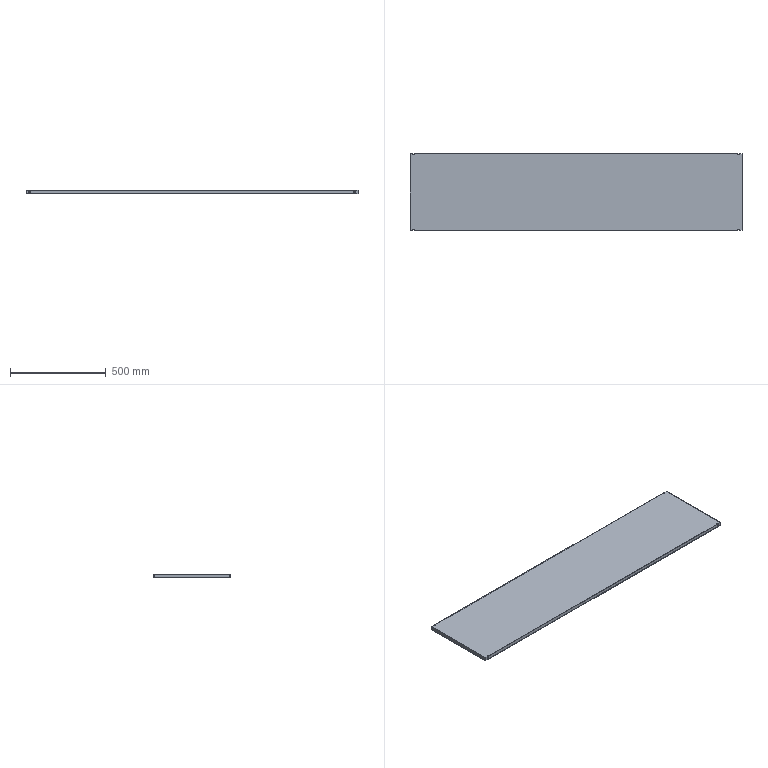Part | SolidWorks | features Extrusion 1, HoleWzd 1, ICE 1, Shell 1 | 1 solid | 40 faces | box 1736 x 400 x 20 mm | volume 1691445 mm3 | plane 32 | cylinder 8 | commonest cylinder face diameters 6.6 x4 11 x4
STEP:
#1=CARTESIAN_POINT('',(-844.877,198.,13.2));
#2=VERTEX_POINT('',#1);
#3=CARTESIAN_POINT('',(-844.877,198.,18.));
#4=VERTEX_POINT('',#3);
#5=CARTESIAN_POINT('',(-844.877,198.,20.));
#6=DIRECTION('',(0.,0.,1.));
#7=VECTOR('',#6,1000.);
#8=LINE('',#5,#7);
#9=EDGE_CURVE('',#2,#4,#8,.T.);
#10=ORIENTED_EDGE('',*,*,#9,.F.);
#11=CARTESIAN_POINT('',(-847.375,198.,13.2));
#12=VERTEX_POINT('',#11);
#13=CARTESIAN_POINT('',(-868.,198.,13.2));
#14=DIRECTION('',(1.,0.,0.));
#15=VECTOR('',#14,1000.);
#16=LINE('',#13,#15);
#17=EDGE_CURVE('',#12,#2,#16,.T.);
#18=ORIENTED_EDGE('',*,*,#17,.F.);
#19=CARTESIAN_POINT('',(-847.375,198.,2.));
#20=VERTEX_POINT('',#19);
#21=CARTESIAN_POINT('',(-847.375,198.,20.));
#22=DIRECTION('',(0.,0.,1.));
#23=VECTOR('',#22,1000.);
#24=LINE('',#21,#23);
#25=EDGE_CURVE('',#20,#12,#24,.T.);
#26=ORIENTED_EDGE('',*,*,#25,.F.);
#27=CARTESIAN_POINT('',(847.375,198.,2.));
#28=VERTEX_POINT('',#27);
#29=CARTESIAN_POINT('',(0.,198.,2.));
#30=DIRECTION('',(-1.,0.,0.));
#31=VECTOR('',#30,1000.);
#32=LINE('',#29,#31);
#33=EDGE_CURVE('',#28,#20,#32,.T.);
#34=ORIENTED_EDGE('',*,*,#33,.F.);
#35=CARTESIAN_POINT('',(847.375,198.,13.2));
#36=VERTEX_POINT('',#35);
#37=CARTESIAN_POINT('',(847.375,198.,20.));
#38=DIRECTION('',(0.,0.,-1.));
#39=VECTOR('',#38,1000.);
#40=LINE('',#37,#39);
#41=EDGE_CURVE('',#36,#28,#40,.T.);
#42=ORIENTED_EDGE('',*,*,#41,.F.);
#43=CARTESIAN_POINT('',(844.877,198.,13.2));
#44=VERTEX_POINT('',#43);
#45=CARTESIAN_POINT('',(-868.,198.,13.2));
#46=DIRECTION('',(1.,0.,0.));
#47=VECTOR('',#46,1000.);
#48=LINE('',#45,#47);
#49=EDGE_CURVE('',#44,#36,#48,.T.);
#50=ORIENTED_EDGE('',*,*,#49,.F.);
#51=CARTESIAN_POINT('',(844.877,198.,18.));
#52=VERTEX_POINT('',#51);
#53=CARTESIAN_POINT('',(844.877,198.,20.));
#54=DIRECTION('',(0.,0.,-1.));
#55=VECTOR('',#54,1000.);
#56=LINE('',#53,#55);
#57=EDGE_CURVE('',#52,#44,#56,.T.);
#58=ORIENTED_EDGE('',*,*,#57,.F.);
#59=CARTESIAN_POINT('',(0.,198.,18.));
#60=DIRECTION('',(-1.,0.,0.));
#61=VECTOR('',#60,1000.);
#62=LINE('',#59,#61);
#63=EDGE_CURVE('',#52,#4,#62,.T.);
#64=ORIENTED_EDGE('',*,*,#63,.T.);
#65=EDGE_LOOP('',(#10,#18,#26,#34,#42,#50,#58,#64));
#66=FACE_OUTER_BOUND('',#65,.T.);
#67=CARTESIAN_POINT('',(-868.,198.,20.));
#68=DIRECTION('',(0.,-1.,0.));
#69=DIRECTION('',(0.,0.,-1.));
#70=AXIS2_PLACEMENT_3D('',#67,#68,#69);
#71=PLANE('',#70);
#72=ADVANCED_FACE('',(#66),#71,.T.);
#73=CARTESIAN_POINT('',(-855.5,200.,20.));
#74=VERTEX_POINT('',#73);
#75=CARTESIAN_POINT('',(-868.,200.,20.));
#76=VERTEX_POINT('',#75);
#77=CARTESIAN_POINT('',(-868.,200.,20.));
#78=DIRECTION('',(-1.,0.,0.));
#79=VECTOR('',#78,1000.);
#80=LINE('',#77,#79);
#81=EDGE_CURVE('',#74,#76,#80,.T.);
#82=ORIENTED_EDGE('',*,*,#81,.F.);
#83=CARTESIAN_POINT('',(-855.5,200.,13.2));
#84=VERTEX_POINT('',#83);
#85=CARTESIAN_POINT('',(-855.5,200.,20.));
#86=DIRECTION('',(0.,0.,-1.));
#87=VECTOR('',#86,1000.);
#88=LINE('',#85,#87);
#89=EDGE_CURVE('',#74,#84,#88,.T.);
#90=ORIENTED_EDGE('',*,*,#89,.T.);
#91=CARTESIAN_POINT('',(-853.3,200.,13.2));
#92=VERTEX_POINT('',#91);
#93=CARTESIAN_POINT('',(-868.,200.,13.2));
#94=DIRECTION('',(1.,0.,0.));
#95=VECTOR('',#94,1000.);
#96=LINE('',#93,#95);
#97=EDGE_CURVE('',#84,#92,#96,.T.);
#98=ORIENTED_EDGE('',*,*,#97,.T.);
#99=CARTESIAN_POINT('',(-853.3,200.,0.));
#100=VERTEX_POINT('',#99);
#101=CARTESIAN_POINT('',(-853.3,200.,20.));
#102=DIRECTION('',(0.,0.,-1.));
#103=VECTOR('',#102,1000.);
#104=LINE('',#101,#103);
#105=EDGE_CURVE('',#92,#100,#104,.T.);
#106=ORIENTED_EDGE('',*,*,#105,.T.);
#107=CARTESIAN_POINT('',(-868.,200.,0.));
#108=VERTEX_POINT('',#107);
#109=CARTESIAN_POINT('',(-868.,200.,0.));
#110=DIRECTION('',(-1.,0.,0.));
#111=VECTOR('',#110,1000.);
#112=LINE('',#109,#111);
#113=EDGE_CURVE('',#100,#108,#112,.T.);
#114=ORIENTED_EDGE('',*,*,#113,.T.);
#115=CARTESIAN_POINT('',(-868.,200.,20.));
#116=DIRECTION('',(0.,0.,-1.));
#117=VECTOR('',#116,1000.);
#118=LINE('',#115,#117);
#119=EDGE_CURVE('',#76,#108,#118,.T.);
#120=ORIENTED_EDGE('',*,*,#119,.F.);
#121=EDGE_LOOP('',(#82,#90,#98,#106,#114,#120));
#122=FACE_OUTER_BOUND('',#121,.T.);
#123=CARTESIAN_POINT('',(-868.,200.,20.));
#124=DIRECTION('',(0.,-1.,0.));
#125=DIRECTION('',(0.,0.,-1.));
#126=AXIS2_PLACEMENT_3D('',#123,#124,#125);
#127=PLANE('',#126);
#128=ADVANCED_FACE('',(#122),#127,.F.);
#129=CARTESIAN_POINT('',(-852.625,-198.,2.));
#130=VERTEX_POINT('',#129);
#131=CARTESIAN_POINT('',(-852.625,-198.,13.2));
#132=VERTEX_POINT('',#131);
#133=CARTESIAN_POINT('',(-852.625,-198.,20.));
#134=DIRECTION('',(0.,0.,1.));
#135=VECTOR('',#134,1000.);
#136=LINE('',#133,#135);
#137=EDGE_CURVE('',#130,#132,#136,.T.);
#138=ORIENTED_EDGE('',*,*,#137,.F.);
#139=CARTESIAN_POINT('',(-866.,-198.,2.));
#140=VERTEX_POINT('',#139);
#141=CARTESIAN_POINT('',(0.,-198.,2.));
#142=DIRECTION('',(1.,0.,0.));
#143=VECTOR('',#142,1000.);
#144=LINE('',#141,#143);
#145=EDGE_CURVE('',#140,#130,#144,.T.);
#146=ORIENTED_EDGE('',*,*,#145,.F.);
#147=CARTESIAN_POINT('',(-866.,-198.,18.));
#148=VERTEX_POINT('',#147);
#149=CARTESIAN_POINT('',(-866.,-198.,20.));
#150=DIRECTION('',(0.,0.,-1.));
#151=VECTOR('',#150,1000.);
#152=LINE('',#149,#151);
#153=EDGE_CURVE('',#148,#140,#152,.T.);
#154=ORIENTED_EDGE('',*,*,#153,.F.);
#155=CARTESIAN_POINT('',(-855.123,-198.,18.));
#156=VERTEX_POINT('',#155);
#157=CARTESIAN_POINT('',(0.,-198.,18.));
#158=DIRECTION('',(1.,0.,0.));
#159=VECTOR('',#158,1000.);
#160=LINE('',#157,#159);
#161=EDGE_CURVE('',#148,#156,#160,.T.);
#162=ORIENTED_EDGE('',*,*,#161,.T.);
#163=CARTESIAN_POINT('',(-855.123,-198.,13.2));
#164=VERTEX_POINT('',#163);
#165=CARTESIAN_POINT('',(-855.123,-198.,20.));
#166=DIRECTION('',(0.,0.,1.));
#167=VECTOR('',#166,1000.);
#168=LINE('',#165,#167);
#169=EDGE_CURVE('',#164,#156,#168,.T.);
#170=ORIENTED_EDGE('',*,*,#169,.F.);
#171=CARTESIAN_POINT('',(-868.,-198.,13.2));
#172=DIRECTION('',(-1.,0.,0.));
#173=VECTOR('',#172,1000.);
#174=LINE('',#171,#173);
#175=EDGE_CURVE('',#132,#164,#174,.T.);
#176=ORIENTED_EDGE('',*,*,#175,.F.);
#177=EDGE_LOOP('',(#138,#146,#154,#162,#170,#176));
#178=FACE_OUTER_BOUND('',#177,.T.);
#179=CARTESIAN_POINT('',(-868.,-198.,20.));
#180=DIRECTION('',(0.,1.,0.));
#181=DIRECTION('',(0.,0.,1.));
#182=AXIS2_PLACEMENT_3D('',#179,#180,#181);
#183=PLANE('',#182);
#184=ADVANCED_FACE('',(#178),#183,.T.);
#185=CARTESIAN_POINT('',(-846.7,200.,0.));
#186=VERTEX_POINT('',#185);
#187=CARTESIAN_POINT('',(-850.,200.,0.));
#188=DIRECTION('',(0.,0.,1.));
#189=DIRECTION('',(1.,0.,0.));
#190=AXIS2_PLACEMENT_3D('',#187,#188,#189);
#191=CIRCLE('',#190,3.3);
#192=EDGE_CURVE('',#100,#186,#191,.T.);
#193=ORIENTED_EDGE('',*,*,#192,.T.);
#194=CARTESIAN_POINT('',(846.7,200.,0.));
#195=VERTEX_POINT('',#194);
#196=CARTESIAN_POINT('',(-868.,200.,0.));
#197=DIRECTION('',(-1.,0.,0.));
#198=VECTOR('',#197,1000.);
#199=LINE('',#196,#198);
#200=EDGE_CURVE('',#195,#186,#199,.T.);
#201=ORIENTED_EDGE('',*,*,#200,.F.);
#202=CARTESIAN_POINT('',(853.3,200.,0.));
#203=VERTEX_POINT('',#202);
#204=CARTESIAN_POINT('',(850.,200.,0.));
#205=DIRECTION('',(0.,0.,1.));
#206=DIRECTION('',(1.,0.,0.));
#207=AXIS2_PLACEMENT_3D('',#204,#205,#206);
#208=CIRCLE('',#207,3.3);
#209=EDGE_CURVE('',#195,#203,#208,.T.);
#210=ORIENTED_EDGE('',*,*,#209,.T.);
#211=CARTESIAN_POINT('',(868.,200.,0.));
#212=VERTEX_POINT('',#211);
#213=CARTESIAN_POINT('',(-868.,200.,0.));
#214=DIRECTION('',(-1.,0.,0.));
#215=VECTOR('',#214,1000.);
#216=LINE('',#213,#215);
#217=EDGE_CURVE('',#212,#203,#216,.T.);
#218=ORIENTED_EDGE('',*,*,#217,.F.);
#219=CARTESIAN_POINT('',(868.,-200.,0.));
#220=VERTEX_POINT('',#219);
#221=CARTESIAN_POINT('',(868.,-200.,0.));
#222=DIRECTION('',(0.,1.,0.));
#223=VECTOR('',#222,1000.);
#224=LINE('',#221,#223);
#225=EDGE_CURVE('',#220,#212,#224,.T.);
#226=ORIENTED_EDGE('',*,*,#225,.F.);
#227=CARTESIAN_POINT('',(853.3,-200.,0.));
#228=VERTEX_POINT('',#227);
#229=CARTESIAN_POINT('',(-868.,-200.,0.));
#230=DIRECTION('',(1.,0.,0.));
#231=VECTOR('',#230,1000.);
#232=LINE('',#229,#231);
#233=EDGE_CURVE('',#228,#220,#232,.T.);
#234=ORIENTED_EDGE('',*,*,#233,.F.);
#235=CARTESIAN_POINT('',(846.7,-200.,0.));
#236=VERTEX_POINT('',#235);
#237=CARTESIAN_POINT('',(850.,-200.,0.));
#238=DIRECTION('',(0.,0.,1.));
#239=DIRECTION('',(1.,0.,0.));
#240=AXIS2_PLACEMENT_3D('',#237,#238,#239);
#241=CIRCLE('',#240,3.3);
#242=EDGE_CURVE('',#228,#236,#241,.T.);
#243=ORIENTED_EDGE('',*,*,#242,.T.);
#244=CARTESIAN_POINT('',(-846.7,-200.,0.));
#245=VERTEX_POINT('',#244);
#246=CARTESIAN_POINT('',(-868.,-200.,0.));
#247=DIRECTION('',(1.,0.,0.));
#248=VECTOR('',#247,1000.);
#249=LINE('',#246,#248);
#250=EDGE_CURVE('',#245,#236,#249,.T.);
#251=ORIENTED_EDGE('',*,*,#250,.F.);
#252=CARTESIAN_POINT('',(-853.3,-200.,0.));
#253=VERTEX_POINT('',#252);
#254=CARTESIAN_POINT('',(-850.,-200.,0.));
#255=DIRECTION('',(0.,0.,1.));
#256=DIRECTION('',(1.,0.,0.));
#257=AXIS2_PLACEMENT_3D('',#254,#255,#256);
#258=CIRCLE('',#257,3.3);
#259=EDGE_CURVE('',#245,#253,#258,.T.);
#260=ORIENTED_EDGE('',*,*,#259,.T.);
#261=CARTESIAN_POINT('',(-868.,-200.,0.));
#262=VERTEX_POINT('',#261);
#263=CARTESIAN_POINT('',(-868.,-200.,0.));
#264=DIRECTION('',(1.,0.,0.));
#265=VECTOR('',#264,1000.);
#266=LINE('',#263,#265);
#267=EDGE_CURVE('',#262,#253,#266,.T.);
#268=ORIENTED_EDGE('',*,*,#267,.F.);
#269=CARTESIAN_POINT('',(-868.,-200.,0.));
#270=DIRECTION('',(0.,-1.,0.));
#271=VECTOR('',#270,1000.);
#272=LINE('',#269,#271);
#273=EDGE_CURVE('',#108,#262,#272,.T.);
#274=ORIENTED_EDGE('',*,*,#273,.F.);
#275=ORIENTED_EDGE('',*,*,#113,.F.);
#276=EDGE_LOOP('',(#193,#201,#210,#218,#226,#234,#243,#251,#260,#268,#274,#275));
#277=FACE_OUTER_BOUND('',#276,.T.);
#278=CARTESIAN_POINT('',(848.,-180.,0.));
#279=VERTEX_POINT('',#278);
#280=CARTESIAN_POINT('',(-848.,-180.,0.));
#281=VERTEX_POINT('',#280);
#282=CARTESIAN_POINT('',(848.,-180.,0.));
#283=DIRECTION('',(-1.,0.,0.));
#284=VECTOR('',#283,1000.);
#285=LINE('',#282,#284);
#286=EDGE_CURVE('',#279,#281,#285,.T.);
#287=ORIENTED_EDGE('',*,*,#286,.F.);
#288=CARTESIAN_POINT('',(848.,180.,0.));
#289=VERTEX_POINT('',#288);
#290=CARTESIAN_POINT('',(848.,-180.,0.));
#291=DIRECTION('',(0.,1.,0.));
#292=VECTOR('',#291,1000.);
#293=LINE('',#290,#292);
#294=EDGE_CURVE('',#279,#289,#293,.T.);
#295=ORIENTED_EDGE('',*,*,#294,.T.);
#296=CARTESIAN_POINT('',(-848.,180.,0.));
#297=VERTEX_POINT('',#296);
#298=CARTESIAN_POINT('',(848.,180.,0.));
#299=DIRECTION('',(-1.,0.,0.));
#300=VECTOR('',#299,1000.);
#301=LINE('',#298,#300);
#302=EDGE_CURVE('',#289,#297,#301,.T.);
#303=ORIENTED_EDGE('',*,*,#302,.T.);
#304=CARTESIAN_POINT('',(-848.,-180.,0.));
#305=DIRECTION('',(0.,1.,0.));
#306=VECTOR('',#305,1000.);
#307=LINE('',#304,#306);
#308=EDGE_CURVE('',#281,#297,#307,.T.);
#309=ORIENTED_EDGE('',*,*,#308,.F.);
#310=EDGE_LOOP('',(#287,#295,#303,#309));
#311=FACE_BOUND('',#310,.T.);
#312=CARTESIAN_POINT('',(0.,0.,0.));
#313=DIRECTION('',(0.,0.,-1.));
#314=DIRECTION('',(-1.,0.,0.));
#315=AXIS2_PLACEMENT_3D('',#312,#313,#314);
#316=PLANE('',#315);
#317=ADVANCED_FACE('',(#277,#311),#316,.T.);
#318=ORIENTED_EDGE('',*,*,#267,.T.);
#319=CARTESIAN_POINT('',(-853.3,-200.,13.2));
#320=VERTEX_POINT('',#319);
#321=CARTESIAN_POINT('',(-853.3,-200.,20.));
#322=DIRECTION('',(0.,0.,1.));
#323=VECTOR('',#322,1000.);
#324=LINE('',#321,#323);
#325=EDGE_CURVE('',#253,#320,#324,.T.);
#326=ORIENTED_EDGE('',*,*,#325,.T.);
#327=CARTESIAN_POINT('',(-855.5,-200.,13.2));
#328=VERTEX_POINT('',#327);
#329=CARTESIAN_POINT('',(-868.,-200.,13.2));
#330=DIRECTION('',(-1.,0.,0.));
#331=VECTOR('',#330,1000.);
#332=LINE('',#329,#331);
#333=EDGE_CURVE('',#320,#328,#332,.T.);
#334=ORIENTED_EDGE('',*,*,#333,.T.);
#335=CARTESIAN_POINT('',(-855.5,-200.,20.));
#336=VERTEX_POINT('',#335);
#337=CARTESIAN_POINT('',(-855.5,-200.,20.));
#338=DIRECTION('',(0.,0.,1.));
#339=VECTOR('',#338,1000.);
#340=LINE('',#337,#339);
#341=EDGE_CURVE('',#328,#336,#340,.T.);
#342=ORIENTED_EDGE('',*,*,#341,.T.);
#343=CARTESIAN_POINT('',(-868.,-200.,20.));
#344=VERTEX_POINT('',#343);
#345=CARTESIAN_POINT('',(-868.,-200.,20.));
#346=DIRECTION('',(1.,0.,0.));
#347=VECTOR('',#346,1000.);
#348=LINE('',#345,#347);
#349=EDGE_CURVE('',#344,#336,#348,.T.);
#350=ORIENTED_EDGE('',*,*,#349,.F.);
#351=CARTESIAN_POINT('',(-868.,-200.,20.));
#352=DIRECTION('',(0.,0.,-1.));
#353=VECTOR('',#352,1000.);
#354=LINE('',#351,#353);
#355=EDGE_CURVE('',#344,#262,#354,.T.);
#356=ORIENTED_EDGE('',*,*,#355,.T.);
#357=EDGE_LOOP('',(#318,#326,#334,#342,#350,#356));
#358=FACE_OUTER_BOUND('',#357,.T.);
#359=CARTESIAN_POINT('',(-868.,-200.,20.));
#360=DIRECTION('',(0.,1.,0.));
#361=DIRECTION('',(0.,0.,1.));
#362=AXIS2_PLACEMENT_3D('',#359,#360,#361);
#363=PLANE('',#362);
#364=ADVANCED_FACE('',(#358),#363,.F.);
#365=CARTESIAN_POINT('',(-844.5,-200.,13.2));
#366=VERTEX_POINT('',#365);
#367=CARTESIAN_POINT('',(-846.7,-200.,13.2));
#368=VERTEX_POINT('',#367);
#369=CARTESIAN_POINT('',(-868.,-200.,13.2));
#370=DIRECTION('',(-1.,0.,0.));
#371=VECTOR('',#370,1000.);
#372=LINE('',#369,#371);
#373=EDGE_CURVE('',#366,#368,#372,.T.);
#374=ORIENTED_EDGE('',*,*,#373,.T.);
#375=CARTESIAN_POINT('',(-846.7,-200.,20.));
#376=DIRECTION('',(0.,0.,-1.));
#377=VECTOR('',#376,1000.);
#378=LINE('',#375,#377);
#379=EDGE_CURVE('',#368,#245,#378,.T.);
#380=ORIENTED_EDGE('',*,*,#379,.T.);
#381=ORIENTED_EDGE('',*,*,#250,.T.);
#382=CARTESIAN_POINT('',(846.7,-200.,13.2));
#383=VERTEX_POINT('',#382);
#384=CARTESIAN_POINT('',(846.7,-200.,20.));
#385=DIRECTION('',(0.,0.,1.));
#386=VECTOR('',#385,1000.);
#387=LINE('',#384,#386);
#388=EDGE_CURVE('',#236,#383,#387,.T.);
#389=ORIENTED_EDGE('',*,*,#388,.T.);
#390=CARTESIAN_POINT('',(844.5,-200.,13.2));
#391=VERTEX_POINT('',#390);
#392=CARTESIAN_POINT('',(-868.,-200.,13.2));
#393=DIRECTION('',(-1.,0.,0.));
#394=VECTOR('',#393,1000.);
#395=LINE('',#392,#394);
#396=EDGE_CURVE('',#383,#391,#395,.T.);
#397=ORIENTED_EDGE('',*,*,#396,.T.);
#398=CARTESIAN_POINT('',(844.5,-200.,20.));
#399=VERTEX_POINT('',#398);
#400=CARTESIAN_POINT('',(844.5,-200.,20.));
#401=DIRECTION('',(0.,0.,1.));
#402=VECTOR('',#401,1000.);
#403=LINE('',#400,#402);
#404=EDGE_CURVE('',#391,#399,#403,.T.);
#405=ORIENTED_EDGE('',*,*,#404,.T.);
#406=CARTESIAN_POINT('',(-844.5,-200.,20.));
#407=VERTEX_POINT('',#406);
#408=CARTESIAN_POINT('',(-868.,-200.,20.));
#409=DIRECTION('',(1.,0.,0.));
#410=VECTOR('',#409,1000.);
#411=LINE('',#408,#410);
#412=EDGE_CURVE('',#407,#399,#411,.T.);
#413=ORIENTED_EDGE('',*,*,#412,.F.);
#414=CARTESIAN_POINT('',(-844.5,-200.,20.));
#415=DIRECTION('',(0.,0.,-1.));
#416=VECTOR('',#415,1000.);
#417=LINE('',#414,#416);
#418=EDGE_CURVE('',#407,#366,#417,.T.);
#419=ORIENTED_EDGE('',*,*,#418,.T.);
#420=EDGE_LOOP('',(#374,#380,#381,#389,#397,#405,#413,#419));
#421=FACE_OUTER_BOUND('',#420,.T.);
#422=CARTESIAN_POINT('',(-868.,-200.,20.));
#423=DIRECTION('',(0.,1.,0.));
#424=DIRECTION('',(0.,0.,1.));
#425=AXIS2_PLACEMENT_3D('',#422,#423,#424);
#426=PLANE('',#425);
#427=ADVANCED_FACE('',(#421),#426,.F.);
#428=CARTESIAN_POINT('',(-847.375,-198.,13.2));
#429=VERTEX_POINT('',#428);
#430=CARTESIAN_POINT('',(-847.375,-198.,2.));
#431=VERTEX_POINT('',#430);
#432=CARTESIAN_POINT('',(-847.375,-198.,20.));
#433=DIRECTION('',(0.,0.,-1.));
#434=VECTOR('',#433,1000.);
#435=LINE('',#432,#434);
#436=EDGE_CURVE('',#429,#431,#435,.T.);
#437=ORIENTED_EDGE('',*,*,#436,.F.);
#438=CARTESIAN_POINT('',(-844.877,-198.,13.2));
#439=VERTEX_POINT('',#438);
#440=CARTESIAN_POINT('',(-868.,-198.,13.2));
#441=DIRECTION('',(-1.,0.,0.));
#442=VECTOR('',#441,1000.);
#443=LINE('',#440,#442);
#444=EDGE_CURVE('',#439,#429,#443,.T.);
#445=ORIENTED_EDGE('',*,*,#444,.F.);
#446=CARTESIAN_POINT('',(-844.877,-198.,18.));
#447=VERTEX_POINT('',#446);
#448=CARTESIAN_POINT('',(-844.877,-198.,20.));
#449=DIRECTION('',(0.,0.,-1.));
#450=VECTOR('',#449,1000.);
#451=LINE('',#448,#450);
#452=EDGE_CURVE('',#447,#439,#451,.T.);
#453=ORIENTED_EDGE('',*,*,#452,.F.);
#454=CARTESIAN_POINT('',(844.877,-198.,18.));
#455=VERTEX_POINT('',#454);
#456=CARTESIAN_POINT('',(0.,-198.,18.));
#457=DIRECTION('',(1.,0.,0.));
#458=VECTOR('',#457,1000.);
#459=LINE('',#456,#458);
#460=EDGE_CURVE('',#447,#455,#459,.T.);
#461=ORIENTED_EDGE('',*,*,#460,.T.);
#462=CARTESIAN_POINT('',(844.877,-198.,13.2));
#463=VERTEX_POINT('',#462);
#464=CARTESIAN_POINT('',(844.877,-198.,20.));
#465=DIRECTION('',(0.,0.,1.));
#466=VECTOR('',#465,1000.);
#467=LINE('',#464,#466);
#468=EDGE_CURVE('',#463,#455,#467,.T.);
#469=ORIENTED_EDGE('',*,*,#468,.F.);
#470=CARTESIAN_POINT('',(847.375,-198.,13.2));
#471=VERTEX_POINT('',#470);
#472=CARTESIAN_POINT('',(-868.,-198.,13.2));
#473=DIRECTION('',(-1.,0.,0.));
#474=VECTOR('',#473,1000.);
#475=LINE('',#472,#474);
#476=EDGE_CURVE('',#471,#463,#475,.T.);
#477=ORIENTED_EDGE('',*,*,#476,.F.);
#478=CARTESIAN_POINT('',(847.375,-198.,2.));
#479=VERTEX_POINT('',#478);
#480=CARTESIAN_POINT('',(847.375,-198.,20.));
#481=DIRECTION('',(0.,0.,1.));
#482=VECTOR('',#481,1000.);
#483=LINE('',#480,#482);
#484=EDGE_CURVE('',#479,#471,#483,.T.);
#485=ORIENTED_EDGE('',*,*,#484,.F.);
#486=CARTESIAN_POINT('',(0.,-198.,2.));
#487=DIRECTION('',(1.,0.,0.));
#488=VECTOR('',#487,1000.);
#489=LINE('',#486,#488);
#490=EDGE_CURVE('',#431,#479,#489,.T.);
#491=ORIENTED_EDGE('',*,*,#490,.F.);
#492=EDGE_LOOP('',(#437,#445,#453,#461,#469,#477,#485,#491));
#493=FACE_OUTER_BOUND('',#492,.T.);
#494=CARTESIAN_POINT('',(-868.,-198.,20.));
#495=DIRECTION('',(0.,1.,0.));
#496=DIRECTION('',(0.,0.,1.));
#497=AXIS2_PLACEMENT_3D('',#494,#495,#496);
#498=PLANE('',#497);
#499=ADVANCED_FACE('',(#493),#498,.T.);
#500=ORIENTED_EDGE('',*,*,#217,.T.);
#501=CARTESIAN_POINT('',(853.3,200.,13.2));
#502=VERTEX_POINT('',#501);
#503=CARTESIAN_POINT('',(853.3,200.,20.));
#504=DIRECTION('',(0.,0.,1.));
#505=VECTOR('',#504,1000.);
#506=LINE('',#503,#505);
#507=EDGE_CURVE('',#203,#502,#506,.T.);
#508=ORIENTED_EDGE('',*,*,#507,.T.);
#509=CARTESIAN_POINT('',(855.5,200.,13.2));
#510=VERTEX_POINT('',#509);
#511=CARTESIAN_POINT('',(-868.,200.,13.2));
#512=DIRECTION('',(1.,0.,0.));
#513=VECTOR('',#512,1000.);
#514=LINE('',#511,#513);
#515=EDGE_CURVE('',#502,#510,#514,.T.);
#516=ORIENTED_EDGE('',*,*,#515,.T.);
#517=CARTESIAN_POINT('',(855.5,200.,20.));
#518=VERTEX_POINT('',#517);
#519=CARTESIAN_POINT('',(855.5,200.,20.));
#520=DIRECTION('',(0.,0.,1.));
#521=VECTOR('',#520,1000.);
#522=LINE('',#519,#521);
#523=EDGE_CURVE('',#510,#518,#522,.T.);
#524=ORIENTED_EDGE('',*,*,#523,.T.);
#525=CARTESIAN_POINT('',(868.,200.,20.));
#526=VERTEX_POINT('',#525);
#527=CARTESIAN_POINT('',(-868.,200.,20.));
#528=DIRECTION('',(-1.,0.,0.));
#529=VECTOR('',#528,1000.);
#530=LINE('',#527,#529);
#531=EDGE_CURVE('',#526,#518,#530,.T.);
#532=ORIENTED_EDGE('',*,*,#531,.F.);
#533=CARTESIAN_POINT('',(868.,200.,20.));
#534=DIRECTION('',(0.,0.,-1.));
#535=VECTOR('',#534,1000.);
#536=LINE('',#533,#535);
#537=EDGE_CURVE('',#526,#212,#536,.T.);
#538=ORIENTED_EDGE('',*,*,#537,.T.);
#539=EDGE_LOOP('',(#500,#508,#516,#524,#532,#538));
#540=FACE_OUTER_BOUND('',#539,.T.);
#541=CARTESIAN_POINT('',(-868.,200.,20.));
#542=DIRECTION('',(0.,-1.,0.));
#543=DIRECTION('',(0.,0.,-1.));
#544=AXIS2_PLACEMENT_3D('',#541,#542,#543);
#545=PLANE('',#544);
#546=ADVANCED_FACE('',(#540),#545,.F.);
#547=CARTESIAN_POINT('',(852.625,198.,2.));
#548=VERTEX_POINT('',#547);
#549=CARTESIAN_POINT('',(852.625,198.,13.2));
#550=VERTEX_POINT('',#549);
#551=CARTESIAN_POINT('',(852.625,198.,20.));
#552=DIRECTION('',(0.,0.,1.));
#553=VECTOR('',#552,1000.);
#554=LINE('',#551,#553);
#555=EDGE_CURVE('',#548,#550,#554,.T.);
#556=ORIENTED_EDGE('',*,*,#555,.F.);
#557=CARTESIAN_POINT('',(866.,198.,2.));
#558=VERTEX_POINT('',#557);
#559=CARTESIAN_POINT('',(0.,198.,2.));
#560=DIRECTION('',(-1.,0.,0.));
#561=VECTOR('',#560,1000.);
#562=LINE('',#559,#561);
#563=EDGE_CURVE('',#558,#548,#562,.T.);
#564=ORIENTED_EDGE('',*,*,#563,.F.);
#565=CARTESIAN_POINT('',(866.,198.,18.));
#566=VERTEX_POINT('',#565);
#567=CARTESIAN_POINT('',(866.,198.,20.));
#568=DIRECTION('',(0.,0.,-1.));
#569=VECTOR('',#568,1000.);
#570=LINE('',#567,#569);
#571=EDGE_CURVE('',#566,#558,#570,.T.);
#572=ORIENTED_EDGE('',*,*,#571,.F.);
#573=CARTESIAN_POINT('',(855.123,198.,18.));
#574=VERTEX_POINT('',#573);
#575=CARTESIAN_POINT('',(0.,198.,18.));
#576=DIRECTION('',(-1.,0.,0.));
#577=VECTOR('',#576,1000.);
#578=LINE('',#575,#577);
#579=EDGE_CURVE('',#566,#574,#578,.T.);
#580=ORIENTED_EDGE('',*,*,#579,.T.);
#581=CARTESIAN_POINT('',(855.123,198.,13.2));
#582=VERTEX_POINT('',#581);
#583=CARTESIAN_POINT('',(855.123,198.,20.));
#584=DIRECTION('',(0.,0.,1.));
#585=VECTOR('',#584,1000.);
#586=LINE('',#583,#585);
#587=EDGE_CURVE('',#582,#574,#586,.T.);
#588=ORIENTED_EDGE('',*,*,#587,.F.);
#589=CARTESIAN_POINT('',(-868.,198.,13.2));
#590=DIRECTION('',(1.,0.,0.));
#591=VECTOR('',#590,1000.);
#592=LINE('',#589,#591);
#593=EDGE_CURVE('',#550,#582,#592,.T.);
#594=ORIENTED_EDGE('',*,*,#593,.F.);
#595=EDGE_LOOP('',(#556,#564,#572,#580,#588,#594));
#596=FACE_OUTER_BOUND('',#595,.T.);
#597=CARTESIAN_POINT('',(-868.,198.,20.));
#598=DIRECTION('',(0.,-1.,0.));
#599=DIRECTION('',(0.,0.,-1.));
#600=AXIS2_PLACEMENT_3D('',#597,#598,#599);
#601=PLANE('',#600);
#602=ADVANCED_FACE('',(#596),#601,.T.);
#603=ORIENTED_EDGE('',*,*,#225,.T.);
#604=ORIENTED_EDGE('',*,*,#537,.F.);
#605=CARTESIAN_POINT('',(868.,-200.,20.));
#606=VERTEX_POINT('',#605);
#607=CARTESIAN_POINT('',(868.,-200.,20.));
#608=DIRECTION('',(0.,1.,0.));
#609=VECTOR('',#608,1000.);
#610=LINE('',#607,#609);
#611=EDGE_CURVE('',#606,#526,#610,.T.);
#612=ORIENTED_EDGE('',*,*,#611,.F.);
#613=CARTESIAN_POINT('',(868.,-200.,20.));
#614=DIRECTION('',(0.,0.,-1.));
#615=VECTOR('',#614,1000.);
#616=LINE('',#613,#615);
#617=EDGE_CURVE('',#606,#220,#616,.T.);
#618=ORIENTED_EDGE('',*,*,#617,.T.);
#619=EDGE_LOOP('',(#603,#604,#612,#618));
#620=FACE_OUTER_BOUND('',#619,.T.);
#621=CARTESIAN_POINT('',(868.,-200.,20.));
#622=DIRECTION('',(-1.,0.,0.));
#623=DIRECTION('',(0.,0.,1.));
#624=AXIS2_PLACEMENT_3D('',#621,#622,#623);
#625=PLANE('',#624);
#626=ADVANCED_FACE('',(#620),#625,.F.);
#627=CARTESIAN_POINT('',(-846.7,200.,13.2));
#628=VERTEX_POINT('',#627);
#629=CARTESIAN_POINT('',(-844.5,200.,13.2));
#630=VERTEX_POINT('',#629);
#631=CARTESIAN_POINT('',(-868.,200.,13.2));
#632=DIRECTION('',(1.,0.,0.));
#633=VECTOR('',#632,1000.);
#634=LINE('',#631,#633);
#635=EDGE_CURVE('',#628,#630,#634,.T.);
#636=ORIENTED_EDGE('',*,*,#635,.T.);
#637=CARTESIAN_POINT('',(-844.5,200.,20.));
#638=VERTEX_POINT('',#637);
#639=CARTESIAN_POINT('',(-844.5,200.,20.));
#640=DIRECTION('',(0.,0.,1.));
#641=VECTOR('',#640,1000.);
#642=LINE('',#639,#641);
#643=EDGE_CURVE('',#630,#638,#642,.T.);
#644=ORIENTED_EDGE('',*,*,#643,.T.);
#645=CARTESIAN_POINT('',(844.5,200.,20.));
#646=VERTEX_POINT('',#645);
#647=CARTESIAN_POINT('',(-868.,200.,20.));
#648=DIRECTION('',(-1.,0.,0.));
#649=VECTOR('',#648,1000.);
#650=LINE('',#647,#649);
#651=EDGE_CURVE('',#646,#638,#650,.T.);
#652=ORIENTED_EDGE('',*,*,#651,.F.);
#653=CARTESIAN_POINT('',(844.5,200.,13.2));
#654=VERTEX_POINT('',#653);
#655=CARTESIAN_POINT('',(844.5,200.,20.));
#656=DIRECTION('',(0.,0.,-1.));
#657=VECTOR('',#656,1000.);
#658=LINE('',#655,#657);
#659=EDGE_CURVE('',#646,#654,#658,.T.);
#660=ORIENTED_EDGE('',*,*,#659,.T.);
#661=CARTESIAN_POINT('',(846.7,200.,13.2));
#662=VERTEX_POINT('',#661);
#663=CARTESIAN_POINT('',(-868.,200.,13.2));
#664=DIRECTION('',(1.,0.,0.));
#665=VECTOR('',#664,1000.);
#666=LINE('',#663,#665);
#667=EDGE_CURVE('',#654,#662,#666,.T.);
#668=ORIENTED_EDGE('',*,*,#667,.T.);
#669=CARTESIAN_POINT('',(846.7,200.,20.));
#670=DIRECTION('',(0.,0.,-1.));
#671=VECTOR('',#670,1000.);
#672=LINE('',#669,#671);
#673=EDGE_CURVE('',#662,#195,#672,.T.);
#674=ORIENTED_EDGE('',*,*,#673,.T.);
#675=ORIENTED_EDGE('',*,*,#200,.T.);
#676=CARTESIAN_POINT('',(-846.7,200.,20.));
#677=DIRECTION('',(0.,0.,1.));
#678=VECTOR('',#677,1000.);
#679=LINE('',#676,#678);
#680=EDGE_CURVE('',#186,#628,#679,.T.);
#681=ORIENTED_EDGE('',*,*,#680,.T.);
#682=EDGE_LOOP('',(#636,#644,#652,#660,#668,#674,#675,#681));
#683=FACE_OUTER_BOUND('',#682,.T.);
#684=CARTESIAN_POINT('',(-868.,200.,20.));
#685=DIRECTION('',(0.,-1.,0.));
#686=DIRECTION('',(0.,0.,-1.));
#687=AXIS2_PLACEMENT_3D('',#684,#685,#686);
#688=PLANE('',#687);
#689=ADVANCED_FACE('',(#683),#688,.F.);
#690=ORIENTED_EDGE('',*,*,#273,.T.);
#691=ORIENTED_EDGE('',*,*,#355,.F.);
#692=CARTESIAN_POINT('',(-868.,-200.,20.));
#693=DIRECTION('',(0.,-1.,0.));
#694=VECTOR('',#693,1000.);
#695=LINE('',#692,#694);
#696=EDGE_CURVE('',#76,#344,#695,.T.);
#697=ORIENTED_EDGE('',*,*,#696,.F.);
#698=ORIENTED_EDGE('',*,*,#119,.T.);
#699=EDGE_LOOP('',(#690,#691,#697,#698));
#700=FACE_OUTER_BOUND('',#699,.T.);
#701=CARTESIAN_POINT('',(-868.,-200.,20.));
#702=DIRECTION('',(1.,0.,0.));
#703=DIRECTION('',(0.,0.,-1.));
#704=AXIS2_PLACEMENT_3D('',#701,#702,#703);
#705=PLANE('',#704);
#706=ADVANCED_FACE('',(#700),#705,.F.);
#707=CARTESIAN_POINT('',(855.5,-200.,20.));
#708=VERTEX_POINT('',#707);
#709=CARTESIAN_POINT('',(-868.,-200.,20.));
#710=DIRECTION('',(1.,0.,0.));
#711=VECTOR('',#710,1000.);
#712=LINE('',#709,#711);
#713=EDGE_CURVE('',#708,#606,#712,.T.);
#714=ORIENTED_EDGE('',*,*,#713,.F.);
#715=CARTESIAN_POINT('',(855.5,-200.,13.2));
#716=VERTEX_POINT('',#715);
#717=CARTESIAN_POINT('',(855.5,-200.,20.));
#718=DIRECTION('',(0.,0.,-1.));
#719=VECTOR('',#718,1000.);
#720=LINE('',#717,#719);
#721=EDGE_CURVE('',#708,#716,#720,.T.);
#722=ORIENTED_EDGE('',*,*,#721,.T.);
#723=CARTESIAN_POINT('',(853.3,-200.,13.2));
#724=VERTEX_POINT('',#723);
#725=CARTESIAN_POINT('',(-868.,-200.,13.2));
#726=DIRECTION('',(-1.,0.,0.));
#727=VECTOR('',#726,1000.);
#728=LINE('',#725,#727);
#729=EDGE_CURVE('',#716,#724,#728,.T.);
#730=ORIENTED_EDGE('',*,*,#729,.T.);
#731=CARTESIAN_POINT('',(853.3,-200.,20.));
#732=DIRECTION('',(0.,0.,-1.));
#733=VECTOR('',#732,1000.);
#734=LINE('',#731,#733);
#735=EDGE_CURVE('',#724,#228,#734,.T.);
#736=ORIENTED_EDGE('',*,*,#735,.T.);
#737=ORIENTED_EDGE('',*,*,#233,.T.);
#738=ORIENTED_EDGE('',*,*,#617,.F.);
#739=EDGE_LOOP('',(#714,#722,#730,#736,#737,#738));
#740=FACE_OUTER_BOUND('',#739,.T.);
#741=CARTESIAN_POINT('',(-868.,-200.,20.));
#742=DIRECTION('',(0.,1.,0.));
#743=DIRECTION('',(0.,0.,1.));
#744=AXIS2_PLACEMENT_3D('',#741,#742,#743);
#745=PLANE('',#744);
#746=ADVANCED_FACE('',(#740),#745,.F.);
#747=ORIENTED_EDGE('',*,*,#651,.T.);
#748=CARTESIAN_POINT('',(-850.,200.,20.));
#749=DIRECTION('',(0.,0.,1.));
#750=DIRECTION('',(1.,0.,0.));
#751=AXIS2_PLACEMENT_3D('',#748,#749,#750);
#752=CIRCLE('',#751,5.5);
#753=EDGE_CURVE('',#74,#638,#752,.T.);
#754=ORIENTED_EDGE('',*,*,#753,.F.);
#755=ORIENTED_EDGE('',*,*,#81,.T.);
#756=ORIENTED_EDGE('',*,*,#696,.T.);
#757=ORIENTED_EDGE('',*,*,#349,.T.);
#758=CARTESIAN_POINT('',(-850.,-200.,20.));
#759=DIRECTION('',(0.,0.,1.));
#760=DIRECTION('',(1.,0.,0.));
#761=AXIS2_PLACEMENT_3D('',#758,#759,#760);
#762=CIRCLE('',#761,5.5);
#763=EDGE_CURVE('',#407,#336,#762,.T.);
#764=ORIENTED_EDGE('',*,*,#763,.F.);
#765=ORIENTED_EDGE('',*,*,#412,.T.);
#766=CARTESIAN_POINT('',(850.,-200.,20.));
#767=DIRECTION('',(0.,0.,1.));
#768=DIRECTION('',(1.,0.,0.));
#769=AXIS2_PLACEMENT_3D('',#766,#767,#768);
#770=CIRCLE('',#769,5.5);
#771=EDGE_CURVE('',#708,#399,#770,.T.);
#772=ORIENTED_EDGE('',*,*,#771,.F.);
#773=ORIENTED_EDGE('',*,*,#713,.T.);
#774=ORIENTED_EDGE('',*,*,#611,.T.);
#775=ORIENTED_EDGE('',*,*,#531,.T.);
#776=CARTESIAN_POINT('',(850.,200.,20.));
#777=DIRECTION('',(0.,0.,1.));
#778=DIRECTION('',(1.,0.,0.));
#779=AXIS2_PLACEMENT_3D('',#776,#777,#778);
#780=CIRCLE('',#779,5.5);
#781=EDGE_CURVE('',#646,#518,#780,.T.);
#782=ORIENTED_EDGE('',*,*,#781,.F.);
#783=EDGE_LOOP('',(#747,#754,#755,#756,#757,#764,#765,#772,#773,#774,#775,#782));
#784=FACE_OUTER_BOUND('',#783,.T.);
#785=CARTESIAN_POINT('',(0.,0.,20.));
#786=DIRECTION('',(0.,0.,-1.));
#787=DIRECTION('',(-1.,0.,0.));
#788=AXIS2_PLACEMENT_3D('',#785,#786,#787);
#789=PLANE('',#788);
#790=ADVANCED_FACE('',(#784),#789,.F.);
#791=ORIENTED_EDGE('',*,*,#294,.F.);
#792=CARTESIAN_POINT('',(848.,-180.,2.));
#793=VERTEX_POINT('',#792);
#794=CARTESIAN_POINT('',(848.,-180.,2.));
#795=DIRECTION('',(0.,0.,-1.));
#796=VECTOR('',#795,1000.);
#797=LINE('',#794,#796);
#798=EDGE_CURVE('',#793,#279,#797,.T.);
#799=ORIENTED_EDGE('',*,*,#798,.F.);
#800=CARTESIAN_POINT('',(848.,180.,2.));
#801=VERTEX_POINT('',#800);
#802=CARTESIAN_POINT('',(848.,-180.,2.));
#803=DIRECTION('',(0.,1.,0.));
#804=VECTOR('',#803,1000.);
#805=LINE('',#802,#804);
#806=EDGE_CURVE('',#793,#801,#805,.T.);
#807=ORIENTED_EDGE('',*,*,#806,.T.);
#808=CARTESIAN_POINT('',(848.,180.,2.));
#809=DIRECTION('',(0.,0.,-1.));
#810=VECTOR('',#809,1000.);
#811=LINE('',#808,#810);
#812=EDGE_CURVE('',#801,#289,#811,.T.);
#813=ORIENTED_EDGE('',*,*,#812,.T.);
#814=EDGE_LOOP('',(#791,#799,#807,#813));
#815=FACE_OUTER_BOUND('',#814,.T.);
#816=CARTESIAN_POINT('',(848.,-180.,2.));
#817=DIRECTION('',(-1.,0.,0.));
#818=DIRECTION('',(0.,0.,1.));
#819=AXIS2_PLACEMENT_3D('',#816,#817,#818);
#820=PLANE('',#819);
#821=ADVANCED_FACE('',(#815),#820,.T.);
#822=ORIENTED_EDGE('',*,*,#302,.F.);
#823=ORIENTED_EDGE('',*,*,#812,.F.);
#824=CARTESIAN_POINT('',(-848.,180.,2.));
#825=VERTEX_POINT('',#824);
#826=CARTESIAN_POINT('',(848.,180.,2.));
#827=DIRECTION('',(-1.,0.,0.));
#828=VECTOR('',#827,1000.);
#829=LINE('',#826,#828);
#830=EDGE_CURVE('',#801,#825,#829,.T.);
#831=ORIENTED_EDGE('',*,*,#830,.T.);
#832=CARTESIAN_POINT('',(-848.,180.,2.));
#833=DIRECTION('',(0.,0.,-1.));
#834=VECTOR('',#833,1000.);
#835=LINE('',#832,#834);
#836=EDGE_CURVE('',#825,#297,#835,.T.);
#837=ORIENTED_EDGE('',*,*,#836,.T.);
#838=EDGE_LOOP('',(#822,#823,#831,#837));
#839=FACE_OUTER_BOUND('',#838,.T.);
#840=CARTESIAN_POINT('',(848.,180.,2.));
#841=DIRECTION('',(0.,-1.,0.));
#842=DIRECTION('',(0.,0.,-1.));
#843=AXIS2_PLACEMENT_3D('',#840,#841,#842);
#844=PLANE('',#843);
#845=ADVANCED_FACE('',(#839),#844,.T.);
#846=ORIENTED_EDGE('',*,*,#308,.T.);
#847=ORIENTED_EDGE('',*,*,#836,.F.);
#848=CARTESIAN_POINT('',(-848.,-180.,2.));
#849=VERTEX_POINT('',#848);
#850=CARTESIAN_POINT('',(-848.,-180.,2.));
#851=DIRECTION('',(0.,1.,0.));
#852=VECTOR('',#851,1000.);
#853=LINE('',#850,#852);
#854=EDGE_CURVE('',#849,#825,#853,.T.);
#855=ORIENTED_EDGE('',*,*,#854,.F.);
#856=CARTESIAN_POINT('',(-848.,-180.,2.));
#857=DIRECTION('',(0.,0.,-1.));
#858=VECTOR('',#857,1000.);
#859=LINE('',#856,#858);
#860=EDGE_CURVE('',#849,#281,#859,.T.);
#861=ORIENTED_EDGE('',*,*,#860,.T.);
#862=EDGE_LOOP('',(#846,#847,#855,#861));
#863=FACE_OUTER_BOUND('',#862,.T.);
#864=CARTESIAN_POINT('',(-848.,-180.,2.));
#865=DIRECTION('',(-1.,0.,0.));
#866=DIRECTION('',(0.,0.,1.));
#867=AXIS2_PLACEMENT_3D('',#864,#865,#866);
#868=PLANE('',#867);
#869=ADVANCED_FACE('',(#863),#868,.F.);
#870=ORIENTED_EDGE('',*,*,#286,.T.);
#871=ORIENTED_EDGE('',*,*,#860,.F.);
#872=CARTESIAN_POINT('',(848.,-180.,2.));
#873=DIRECTION('',(-1.,0.,0.));
#874=VECTOR('',#873,1000.);
#875=LINE('',#872,#874);
#876=EDGE_CURVE('',#793,#849,#875,.T.);
#877=ORIENTED_EDGE('',*,*,#876,.F.);
#878=ORIENTED_EDGE('',*,*,#798,.T.);
#879=EDGE_LOOP('',(#870,#871,#877,#878));
#880=FACE_OUTER_BOUND('',#879,.T.);
#881=CARTESIAN_POINT('',(848.,-180.,2.));
#882=DIRECTION('',(0.,-1.,0.));
#883=DIRECTION('',(0.,0.,-1.));
#884=AXIS2_PLACEMENT_3D('',#881,#882,#883);
#885=PLANE('',#884);
#886=ADVANCED_FACE('',(#880),#885,.F.);
#887=ORIENTED_EDGE('',*,*,#33,.T.);
#888=CARTESIAN_POINT('',(-852.625,198.,2.));
#889=VERTEX_POINT('',#888);
#890=CARTESIAN_POINT('',(-850.,200.,2.));
#891=DIRECTION('',(0.,0.,-1.));
#892=DIRECTION('',(-1.,0.,0.));
#893=AXIS2_PLACEMENT_3D('',#890,#891,#892);
#894=CIRCLE('',#893,3.3);
#895=EDGE_CURVE('',#20,#889,#894,.T.);
#896=ORIENTED_EDGE('',*,*,#895,.T.);
#897=CARTESIAN_POINT('',(-866.,198.,2.));
#898=VERTEX_POINT('',#897);
#899=CARTESIAN_POINT('',(0.,198.,2.));
#900=DIRECTION('',(-1.,0.,0.));
#901=VECTOR('',#900,1000.);
#902=LINE('',#899,#901);
#903=EDGE_CURVE('',#889,#898,#902,.T.);
#904=ORIENTED_EDGE('',*,*,#903,.T.);
#905=CARTESIAN_POINT('',(-866.,0.,2.));
#906=DIRECTION('',(0.,-1.,0.));
#907=VECTOR('',#906,1000.);
#908=LINE('',#905,#907);
#909=EDGE_CURVE('',#898,#140,#908,.T.);
#910=ORIENTED_EDGE('',*,*,#909,.T.);
#911=ORIENTED_EDGE('',*,*,#145,.T.);
#912=CARTESIAN_POINT('',(-850.,-200.,2.));
#913=DIRECTION('',(0.,0.,-1.));
#914=DIRECTION('',(-1.,0.,0.));
#915=AXIS2_PLACEMENT_3D('',#912,#913,#914);
#916=CIRCLE('',#915,3.3);
#917=EDGE_CURVE('',#130,#431,#916,.T.);
#918=ORIENTED_EDGE('',*,*,#917,.T.);
#919=ORIENTED_EDGE('',*,*,#490,.T.);
#920=CARTESIAN_POINT('',(852.625,-198.,2.));
#921=VERTEX_POINT('',#920);
#922=CARTESIAN_POINT('',(850.,-200.,2.));
#923=DIRECTION('',(0.,0.,-1.));
#924=DIRECTION('',(-1.,0.,0.));
#925=AXIS2_PLACEMENT_3D('',#922,#923,#924);
#926=CIRCLE('',#925,3.3);
#927=EDGE_CURVE('',#479,#921,#926,.T.);
#928=ORIENTED_EDGE('',*,*,#927,.T.);
#929=CARTESIAN_POINT('',(866.,-198.,2.));
#930=VERTEX_POINT('',#929);
#931=CARTESIAN_POINT('',(0.,-198.,2.));
#932=DIRECTION('',(1.,0.,0.));
#933=VECTOR('',#932,1000.);
#934=LINE('',#931,#933);
#935=EDGE_CURVE('',#921,#930,#934,.T.);
#936=ORIENTED_EDGE('',*,*,#935,.T.);
#937=CARTESIAN_POINT('',(866.,0.,2.));
#938=DIRECTION('',(0.,1.,0.));
#939=VECTOR('',#938,1000.);
#940=LINE('',#937,#939);
#941=EDGE_CURVE('',#930,#558,#940,.T.);
#942=ORIENTED_EDGE('',*,*,#941,.T.);
#943=ORIENTED_EDGE('',*,*,#563,.T.);
#944=CARTESIAN_POINT('',(850.,200.,2.));
#945=DIRECTION('',(0.,0.,-1.));
#946=DIRECTION('',(-1.,0.,0.));
#947=AXIS2_PLACEMENT_3D('',#944,#945,#946);
#948=CIRCLE('',#947,3.3);
#949=EDGE_CURVE('',#548,#28,#948,.T.);
#950=ORIENTED_EDGE('',*,*,#949,.T.);
#951=EDGE_LOOP('',(#887,#896,#904,#910,#911,#918,#919,#928,#936,#942,#943,#950));
#952=FACE_OUTER_BOUND('',#951,.T.);
#953=ORIENTED_EDGE('',*,*,#876,.T.);
#954=ORIENTED_EDGE('',*,*,#854,.T.);
#955=ORIENTED_EDGE('',*,*,#830,.F.);
#956=ORIENTED_EDGE('',*,*,#806,.F.);
#957=EDGE_LOOP('',(#953,#954,#955,#956));
#958=FACE_BOUND('',#957,.T.);
#959=CARTESIAN_POINT('',(0.,0.,2.));
#960=DIRECTION('',(0.,0.,-1.));
#961=DIRECTION('',(-1.,0.,0.));
#962=AXIS2_PLACEMENT_3D('',#959,#960,#961);
#963=PLANE('',#962);
#964=ADVANCED_FACE('',(#952,#958),#963,.F.);
#965=ORIENTED_EDGE('',*,*,#941,.F.);
#966=CARTESIAN_POINT('',(866.,-198.,18.));
#967=VERTEX_POINT('',#966);
#968=CARTESIAN_POINT('',(866.,-198.,20.));
#969=DIRECTION('',(0.,0.,-1.));
#970=VECTOR('',#969,1000.);
#971=LINE('',#968,#970);
#972=EDGE_CURVE('',#967,#930,#971,.T.);
#973=ORIENTED_EDGE('',*,*,#972,.F.);
#974=CARTESIAN_POINT('',(866.,0.,18.));
#975=DIRECTION('',(0.,1.,0.));
#976=VECTOR('',#975,1000.);
#977=LINE('',#974,#976);
#978=EDGE_CURVE('',#967,#566,#977,.T.);
#979=ORIENTED_EDGE('',*,*,#978,.T.);
#980=ORIENTED_EDGE('',*,*,#571,.T.);
#981=EDGE_LOOP('',(#965,#973,#979,#980));
#982=FACE_OUTER_BOUND('',#981,.T.);
#983=CARTESIAN_POINT('',(866.,-200.,20.));
#984=DIRECTION('',(-1.,0.,0.));
#985=DIRECTION('',(0.,0.,1.));
#986=AXIS2_PLACEMENT_3D('',#983,#984,#985);
#987=PLANE('',#986);
#988=ADVANCED_FACE('',(#982),#987,.T.);
#989=CARTESIAN_POINT('',(-855.123,198.,18.));
#990=VERTEX_POINT('',#989);
#991=CARTESIAN_POINT('',(-855.123,198.,13.2));
#992=VERTEX_POINT('',#991);
#993=CARTESIAN_POINT('',(-855.123,198.,20.));
#994=DIRECTION('',(0.,0.,-1.));
#995=VECTOR('',#994,1000.);
#996=LINE('',#993,#995);
#997=EDGE_CURVE('',#990,#992,#996,.T.);
#998=ORIENTED_EDGE('',*,*,#997,.F.);
#999=CARTESIAN_POINT('',(-866.,198.,18.));
#1000=VERTEX_POINT('',#999);
#1001=CARTESIAN_POINT('',(0.,198.,18.));
#1002=DIRECTION('',(-1.,0.,0.));
#1003=VECTOR('',#1002,1000.);
#1004=LINE('',#1001,#1003);
#1005=EDGE_CURVE('',#990,#1000,#1004,.T.);
#1006=ORIENTED_EDGE('',*,*,#1005,.T.);
#1007=CARTESIAN_POINT('',(-866.,198.,20.));
#1008=DIRECTION('',(0.,0.,-1.));
#1009=VECTOR('',#1008,1000.);
#1010=LINE('',#1007,#1009);
#1011=EDGE_CURVE('',#1000,#898,#1010,.T.);
#1012=ORIENTED_EDGE('',*,*,#1011,.T.);
#1013=ORIENTED_EDGE('',*,*,#903,.F.);
#1014=CARTESIAN_POINT('',(-852.625,198.,13.2));
#1015=VERTEX_POINT('',#1014);
#1016=CARTESIAN_POINT('',(-852.625,198.,20.));
#1017=DIRECTION('',(0.,0.,-1.));
#1018=VECTOR('',#1017,1000.);
#1019=LINE('',#1016,#1018);
#1020=EDGE_CURVE('',#1015,#889,#1019,.T.);
#1021=ORIENTED_EDGE('',*,*,#1020,.F.);
#1022=CARTESIAN_POINT('',(-868.,198.,13.2));
#1023=DIRECTION('',(1.,0.,0.));
#1024=VECTOR('',#1023,1000.);
#1025=LINE('',#1022,#1024);
#1026=EDGE_CURVE('',#992,#1015,#1025,.T.);
#1027=ORIENTED_EDGE('',*,*,#1026,.F.);
#1028=EDGE_LOOP('',(#998,#1006,#1012,#1013,#1021,#1027));
#1029=FACE_OUTER_BOUND('',#1028,.T.);
#1030=CARTESIAN_POINT('',(-868.,198.,20.));
#1031=DIRECTION('',(0.,-1.,0.));
#1032=DIRECTION('',(0.,0.,-1.));
#1033=AXIS2_PLACEMENT_3D('',#1030,#1031,#1032);
#1034=PLANE('',#1033);
#1035=ADVANCED_FACE('',(#1029),#1034,.T.);
#1036=ORIENTED_EDGE('',*,*,#909,.F.);
#1037=ORIENTED_EDGE('',*,*,#1011,.F.);
#1038=CARTESIAN_POINT('',(-866.,0.,18.));
#1039=DIRECTION('',(0.,-1.,0.));
#1040=VECTOR('',#1039,1000.);
#1041=LINE('',#1038,#1040);
#1042=EDGE_CURVE('',#1000,#148,#1041,.T.);
#1043=ORIENTED_EDGE('',*,*,#1042,.T.);
#1044=ORIENTED_EDGE('',*,*,#153,.T.);
#1045=EDGE_LOOP('',(#1036,#1037,#1043,#1044));
#1046=FACE_OUTER_BOUND('',#1045,.T.);
#1047=CARTESIAN_POINT('',(-866.,-200.,20.));
#1048=DIRECTION('',(1.,0.,0.));
#1049=DIRECTION('',(0.,0.,-1.));
#1050=AXIS2_PLACEMENT_3D('',#1047,#1048,#1049);
#1051=PLANE('',#1050);
#1052=ADVANCED_FACE('',(#1046),#1051,.T.);
#1053=CARTESIAN_POINT('',(852.625,-198.,13.2));
#1054=VERTEX_POINT('',#1053);
#1055=CARTESIAN_POINT('',(852.625,-198.,20.));
#1056=DIRECTION('',(0.,0.,-1.));
#1057=VECTOR('',#1056,1000.);
#1058=LINE('',#1055,#1057);
#1059=EDGE_CURVE('',#1054,#921,#1058,.T.);
#1060=ORIENTED_EDGE('',*,*,#1059,.F.);
#1061=CARTESIAN_POINT('',(855.123,-198.,13.2));
#1062=VERTEX_POINT('',#1061);
#1063=CARTESIAN_POINT('',(-868.,-198.,13.2));
#1064=DIRECTION('',(-1.,0.,0.));
#1065=VECTOR('',#1064,1000.);
#1066=LINE('',#1063,#1065);
#1067=EDGE_CURVE('',#1062,#1054,#1066,.T.);
#1068=ORIENTED_EDGE('',*,*,#1067,.F.);
#1069=CARTESIAN_POINT('',(855.123,-198.,18.));
#1070=VERTEX_POINT('',#1069);
#1071=CARTESIAN_POINT('',(855.123,-198.,20.));
#1072=DIRECTION('',(0.,0.,-1.));
#1073=VECTOR('',#1072,1000.);
#1074=LINE('',#1071,#1073);
#1075=EDGE_CURVE('',#1070,#1062,#1074,.T.);
#1076=ORIENTED_EDGE('',*,*,#1075,.F.);
#1077=CARTESIAN_POINT('',(0.,-198.,18.));
#1078=DIRECTION('',(1.,0.,0.));
#1079=VECTOR('',#1078,1000.);
#1080=LINE('',#1077,#1079);
#1081=EDGE_CURVE('',#1070,#967,#1080,.T.);
#1082=ORIENTED_EDGE('',*,*,#1081,.T.);
#1083=ORIENTED_EDGE('',*,*,#972,.T.);
#1084=ORIENTED_EDGE('',*,*,#935,.F.);
#1085=EDGE_LOOP('',(#1060,#1068,#1076,#1082,#1083,#1084));
#1086=FACE_OUTER_BOUND('',#1085,.T.);
#1087=CARTESIAN_POINT('',(-868.,-198.,20.));
#1088=DIRECTION('',(0.,1.,0.));
#1089=DIRECTION('',(0.,0.,1.));
#1090=AXIS2_PLACEMENT_3D('',#1087,#1088,#1089);
#1091=PLANE('',#1090);
#1092=ADVANCED_FACE('',(#1086),#1091,.T.);
#1093=CARTESIAN_POINT('',(-850.,200.,18.));
#1094=DIRECTION('',(0.,0.,-1.));
#1095=DIRECTION('',(-1.,0.,0.));
#1096=AXIS2_PLACEMENT_3D('',#1093,#1094,#1095);
#1097=CIRCLE('',#1096,5.5);
#1098=EDGE_CURVE('',#4,#990,#1097,.T.);
#1099=ORIENTED_EDGE('',*,*,#1098,.F.);
#1100=ORIENTED_EDGE('',*,*,#63,.F.);
#1101=CARTESIAN_POINT('',(850.,200.,18.));
#1102=DIRECTION('',(0.,0.,-1.));
#1103=DIRECTION('',(-1.,0.,0.));
#1104=AXIS2_PLACEMENT_3D('',#1101,#1102,#1103);
#1105=CIRCLE('',#1104,5.5);
#1106=EDGE_CURVE('',#574,#52,#1105,.T.);
#1107=ORIENTED_EDGE('',*,*,#1106,.F.);
#1108=ORIENTED_EDGE('',*,*,#579,.F.);
#1109=ORIENTED_EDGE('',*,*,#978,.F.);
#1110=ORIENTED_EDGE('',*,*,#1081,.F.);
#1111=CARTESIAN_POINT('',(850.,-200.,18.));
#1112=DIRECTION('',(0.,0.,-1.));
#1113=DIRECTION('',(-1.,0.,0.));
#1114=AXIS2_PLACEMENT_3D('',#1111,#1112,#1113);
#1115=CIRCLE('',#1114,5.5);
#1116=EDGE_CURVE('',#455,#1070,#1115,.T.);
#1117=ORIENTED_EDGE('',*,*,#1116,.F.);
#1118=ORIENTED_EDGE('',*,*,#460,.F.);
#1119=CARTESIAN_POINT('',(-850.,-200.,18.));
#1120=DIRECTION('',(0.,0.,-1.));
#1121=DIRECTION('',(-1.,0.,0.));
#1122=AXIS2_PLACEMENT_3D('',#1119,#1120,#1121);
#1123=CIRCLE('',#1122,5.5);
#1124=EDGE_CURVE('',#156,#447,#1123,.T.);
#1125=ORIENTED_EDGE('',*,*,#1124,.F.);
#1126=ORIENTED_EDGE('',*,*,#161,.F.);
#1127=ORIENTED_EDGE('',*,*,#1042,.F.);
#1128=ORIENTED_EDGE('',*,*,#1005,.F.);
#1129=EDGE_LOOP('',(#1099,#1100,#1107,#1108,#1109,#1110,#1117,#1118,#1125,#1126,#1127,#1128));
#1130=FACE_OUTER_BOUND('',#1129,.T.);
#1131=CARTESIAN_POINT('',(0.,0.,18.));
#1132=DIRECTION('',(0.,0.,-1.));
#1133=DIRECTION('',(-1.,0.,0.));
#1134=AXIS2_PLACEMENT_3D('',#1131,#1132,#1133);
#1135=PLANE('',#1134);
#1136=ADVANCED_FACE('',(#1130),#1135,.T.);
#1137=CARTESIAN_POINT('',(850.,200.,13.2));
#1138=DIRECTION('',(0.,0.,1.));
#1139=DIRECTION('',(1.,0.,0.));
#1140=AXIS2_PLACEMENT_3D('',#1137,#1138,#1139);
#1141=CIRCLE('',#1140,5.5);
#1142=EDGE_CURVE('',#654,#44,#1141,.T.);
#1143=ORIENTED_EDGE('',*,*,#1142,.T.);
#1144=ORIENTED_EDGE('',*,*,#49,.T.);
#1145=CARTESIAN_POINT('',(850.,200.,13.2));
#1146=DIRECTION('',(0.,0.,1.));
#1147=DIRECTION('',(1.,0.,0.));
#1148=AXIS2_PLACEMENT_3D('',#1145,#1146,#1147);
#1149=CIRCLE('',#1148,3.3);
#1150=EDGE_CURVE('',#662,#36,#1149,.T.);
#1151=ORIENTED_EDGE('',*,*,#1150,.F.);
#1152=ORIENTED_EDGE('',*,*,#667,.F.);
#1153=EDGE_LOOP('',(#1143,#1144,#1151,#1152));
#1154=FACE_OUTER_BOUND('',#1153,.T.);
#1155=CARTESIAN_POINT('',(853.3,200.,13.2));
#1156=DIRECTION('',(0.,0.,-1.));
#1157=DIRECTION('',(-1.,0.,0.));
#1158=AXIS2_PLACEMENT_3D('',#1155,#1156,#1157);
#1159=PLANE('',#1158);
#1160=ADVANCED_FACE('',(#1154),#1159,.F.);
#1161=CARTESIAN_POINT('',(850.,200.,13.2));
#1162=DIRECTION('',(0.,0.,1.));
#1163=DIRECTION('',(1.,0.,0.));
#1164=AXIS2_PLACEMENT_3D('',#1161,#1162,#1163);
#1165=CIRCLE('',#1164,3.3);
#1166=EDGE_CURVE('',#550,#502,#1165,.T.);
#1167=ORIENTED_EDGE('',*,*,#1166,.F.);
#1168=ORIENTED_EDGE('',*,*,#593,.T.);
#1169=CARTESIAN_POINT('',(850.,200.,13.2));
#1170=DIRECTION('',(0.,0.,1.));
#1171=DIRECTION('',(1.,0.,0.));
#1172=AXIS2_PLACEMENT_3D('',#1169,#1170,#1171);
#1173=CIRCLE('',#1172,5.5);
#1174=EDGE_CURVE('',#582,#510,#1173,.T.);
#1175=ORIENTED_EDGE('',*,*,#1174,.T.);
#1176=ORIENTED_EDGE('',*,*,#515,.F.);
#1177=EDGE_LOOP('',(#1167,#1168,#1175,#1176));
#1178=FACE_OUTER_BOUND('',#1177,.T.);
#1179=CARTESIAN_POINT('',(853.3,200.,13.2));
#1180=DIRECTION('',(0.,0.,-1.));
#1181=DIRECTION('',(-1.,0.,0.));
#1182=AXIS2_PLACEMENT_3D('',#1179,#1180,#1181);
#1183=PLANE('',#1182);
#1184=ADVANCED_FACE('',(#1178),#1183,.F.);
#1185=ORIENTED_EDGE('',*,*,#209,.F.);
#1186=ORIENTED_EDGE('',*,*,#673,.F.);
#1187=ORIENTED_EDGE('',*,*,#1150,.T.);
#1188=ORIENTED_EDGE('',*,*,#41,.T.);
#1189=ORIENTED_EDGE('',*,*,#949,.F.);
#1190=ORIENTED_EDGE('',*,*,#555,.T.);
#1191=ORIENTED_EDGE('',*,*,#1166,.T.);
#1192=ORIENTED_EDGE('',*,*,#507,.F.);
#1193=EDGE_LOOP('',(#1185,#1186,#1187,#1188,#1189,#1190,#1191,#1192));
#1194=FACE_OUTER_BOUND('',#1193,.T.);
#1195=CARTESIAN_POINT('',(850.,200.,20.));
#1196=DIRECTION('',(0.,0.,1.));
#1197=DIRECTION('',(1.,0.,0.));
#1198=AXIS2_PLACEMENT_3D('',#1195,#1196,#1197);
#1199=CYLINDRICAL_SURFACE('',#1198,3.3);
#1200=ADVANCED_FACE('',(#1194),#1199,.F.);
#1201=ORIENTED_EDGE('',*,*,#1174,.F.);
#1202=ORIENTED_EDGE('',*,*,#587,.T.);
#1203=ORIENTED_EDGE('',*,*,#1106,.T.);
#1204=ORIENTED_EDGE('',*,*,#57,.T.);
#1205=ORIENTED_EDGE('',*,*,#1142,.F.);
#1206=ORIENTED_EDGE('',*,*,#659,.F.);
#1207=ORIENTED_EDGE('',*,*,#781,.T.);
#1208=ORIENTED_EDGE('',*,*,#523,.F.);
#1209=EDGE_LOOP('',(#1201,#1202,#1203,#1204,#1205,#1206,#1207,#1208));
#1210=FACE_OUTER_BOUND('',#1209,.T.);
#1211=CARTESIAN_POINT('',(850.,200.,20.));
#1212=DIRECTION('',(0.,0.,1.));
#1213=DIRECTION('',(1.,0.,0.));
#1214=AXIS2_PLACEMENT_3D('',#1211,#1212,#1213);
#1215=CYLINDRICAL_SURFACE('',#1214,5.5);
#1216=ADVANCED_FACE('',(#1210),#1215,.F.);
#1217=CARTESIAN_POINT('',(850.,-200.,13.2));
#1218=DIRECTION('',(0.,0.,1.));
#1219=DIRECTION('',(1.,0.,0.));
#1220=AXIS2_PLACEMENT_3D('',#1217,#1218,#1219);
#1221=CIRCLE('',#1220,5.5);
#1222=EDGE_CURVE('',#716,#1062,#1221,.T.);
#1223=ORIENTED_EDGE('',*,*,#1222,.T.);
#1224=ORIENTED_EDGE('',*,*,#1067,.T.);
#1225=CARTESIAN_POINT('',(850.,-200.,13.2));
#1226=DIRECTION('',(0.,0.,1.));
#1227=DIRECTION('',(1.,0.,0.));
#1228=AXIS2_PLACEMENT_3D('',#1225,#1226,#1227);
#1229=CIRCLE('',#1228,3.3);
#1230=EDGE_CURVE('',#724,#1054,#1229,.T.);
#1231=ORIENTED_EDGE('',*,*,#1230,.F.);
#1232=ORIENTED_EDGE('',*,*,#729,.F.);
#1233=EDGE_LOOP('',(#1223,#1224,#1231,#1232));
#1234=FACE_OUTER_BOUND('',#1233,.T.);
#1235=CARTESIAN_POINT('',(853.3,-200.,13.2));
#1236=DIRECTION('',(0.,0.,-1.));
#1237=DIRECTION('',(-1.,0.,0.));
#1238=AXIS2_PLACEMENT_3D('',#1235,#1236,#1237);
#1239=PLANE('',#1238);
#1240=ADVANCED_FACE('',(#1234),#1239,.F.);
#1241=CARTESIAN_POINT('',(850.,-200.,13.2));
#1242=DIRECTION('',(0.,0.,1.));
#1243=DIRECTION('',(1.,0.,0.));
#1244=AXIS2_PLACEMENT_3D('',#1241,#1242,#1243);
#1245=CIRCLE('',#1244,3.3);
#1246=EDGE_CURVE('',#471,#383,#1245,.T.);
#1247=ORIENTED_EDGE('',*,*,#1246,.F.);
#1248=ORIENTED_EDGE('',*,*,#476,.T.);
#1249=CARTESIAN_POINT('',(850.,-200.,13.2));
#1250=DIRECTION('',(0.,0.,1.));
#1251=DIRECTION('',(1.,0.,0.));
#1252=AXIS2_PLACEMENT_3D('',#1249,#1250,#1251);
#1253=CIRCLE('',#1252,5.5);
#1254=EDGE_CURVE('',#463,#391,#1253,.T.);
#1255=ORIENTED_EDGE('',*,*,#1254,.T.);
#1256=ORIENTED_EDGE('',*,*,#396,.F.);
#1257=EDGE_LOOP('',(#1247,#1248,#1255,#1256));
#1258=FACE_OUTER_BOUND('',#1257,.T.);
#1259=CARTESIAN_POINT('',(853.3,-200.,13.2));
#1260=DIRECTION('',(0.,0.,-1.));
#1261=DIRECTION('',(-1.,0.,0.));
#1262=AXIS2_PLACEMENT_3D('',#1259,#1260,#1261);
#1263=PLANE('',#1262);
#1264=ADVANCED_FACE('',(#1258),#1263,.F.);
#1265=ORIENTED_EDGE('',*,*,#242,.F.);
#1266=ORIENTED_EDGE('',*,*,#735,.F.);
#1267=ORIENTED_EDGE('',*,*,#1230,.T.);
#1268=ORIENTED_EDGE('',*,*,#1059,.T.);
#1269=ORIENTED_EDGE('',*,*,#927,.F.);
#1270=ORIENTED_EDGE('',*,*,#484,.T.);
#1271=ORIENTED_EDGE('',*,*,#1246,.T.);
#1272=ORIENTED_EDGE('',*,*,#388,.F.);
#1273=EDGE_LOOP('',(#1265,#1266,#1267,#1268,#1269,#1270,#1271,#1272));
#1274=FACE_OUTER_BOUND('',#1273,.T.);
#1275=CARTESIAN_POINT('',(850.,-200.,20.));
#1276=DIRECTION('',(0.,0.,1.));
#1277=DIRECTION('',(1.,0.,0.));
#1278=AXIS2_PLACEMENT_3D('',#1275,#1276,#1277);
#1279=CYLINDRICAL_SURFACE('',#1278,3.3);
#1280=ADVANCED_FACE('',(#1274),#1279,.F.);
#1281=ORIENTED_EDGE('',*,*,#1254,.F.);
#1282=ORIENTED_EDGE('',*,*,#468,.T.);
#1283=ORIENTED_EDGE('',*,*,#1116,.T.);
#1284=ORIENTED_EDGE('',*,*,#1075,.T.);
#1285=ORIENTED_EDGE('',*,*,#1222,.F.);
#1286=ORIENTED_EDGE('',*,*,#721,.F.);
#1287=ORIENTED_EDGE('',*,*,#771,.T.);
#1288=ORIENTED_EDGE('',*,*,#404,.F.);
#1289=EDGE_LOOP('',(#1281,#1282,#1283,#1284,#1285,#1286,#1287,#1288));
#1290=FACE_OUTER_BOUND('',#1289,.T.);
#1291=CARTESIAN_POINT('',(850.,-200.,20.));
#1292=DIRECTION('',(0.,0.,1.));
#1293=DIRECTION('',(1.,0.,0.));
#1294=AXIS2_PLACEMENT_3D('',#1291,#1292,#1293);
#1295=CYLINDRICAL_SURFACE('',#1294,5.5);
#1296=ADVANCED_FACE('',(#1290),#1295,.F.);
#1297=ORIENTED_EDGE('',*,*,#444,.T.);
#1298=CARTESIAN_POINT('',(-850.,-200.,13.2));
#1299=DIRECTION('',(0.,0.,1.));
#1300=DIRECTION('',(1.,0.,0.));
#1301=AXIS2_PLACEMENT_3D('',#1298,#1299,#1300);
#1302=CIRCLE('',#1301,3.3);
#1303=EDGE_CURVE('',#368,#429,#1302,.T.);
#1304=ORIENTED_EDGE('',*,*,#1303,.F.);
#1305=ORIENTED_EDGE('',*,*,#373,.F.);
#1306=CARTESIAN_POINT('',(-850.,-200.,13.2));
#1307=DIRECTION('',(0.,0.,1.));
#1308=DIRECTION('',(1.,0.,0.));
#1309=AXIS2_PLACEMENT_3D('',#1306,#1307,#1308);
#1310=CIRCLE('',#1309,5.5);
#1311=EDGE_CURVE('',#366,#439,#1310,.T.);
#1312=ORIENTED_EDGE('',*,*,#1311,.T.);
#1313=EDGE_LOOP('',(#1297,#1304,#1305,#1312));
#1314=FACE_OUTER_BOUND('',#1313,.T.);
#1315=CARTESIAN_POINT('',(-846.7,-200.,13.2));
#1316=DIRECTION('',(0.,0.,-1.));
#1317=DIRECTION('',(-1.,0.,0.));
#1318=AXIS2_PLACEMENT_3D('',#1315,#1316,#1317);
#1319=PLANE('',#1318);
#1320=ADVANCED_FACE('',(#1314),#1319,.F.);
#1321=ORIENTED_EDGE('',*,*,#175,.T.);
#1322=CARTESIAN_POINT('',(-850.,-200.,13.2));
#1323=DIRECTION('',(0.,0.,1.));
#1324=DIRECTION('',(1.,0.,0.));
#1325=AXIS2_PLACEMENT_3D('',#1322,#1323,#1324);
#1326=CIRCLE('',#1325,5.5);
#1327=EDGE_CURVE('',#164,#328,#1326,.T.);
#1328=ORIENTED_EDGE('',*,*,#1327,.T.);
#1329=ORIENTED_EDGE('',*,*,#333,.F.);
#1330=CARTESIAN_POINT('',(-850.,-200.,13.2));
#1331=DIRECTION('',(0.,0.,1.));
#1332=DIRECTION('',(1.,0.,0.));
#1333=AXIS2_PLACEMENT_3D('',#1330,#1331,#1332);
#1334=CIRCLE('',#1333,3.3);
#1335=EDGE_CURVE('',#132,#320,#1334,.T.);
#1336=ORIENTED_EDGE('',*,*,#1335,.F.);
#1337=EDGE_LOOP('',(#1321,#1328,#1329,#1336));
#1338=FACE_OUTER_BOUND('',#1337,.T.);
#1339=CARTESIAN_POINT('',(-846.7,-200.,13.2));
#1340=DIRECTION('',(0.,0.,-1.));
#1341=DIRECTION('',(-1.,0.,0.));
#1342=AXIS2_PLACEMENT_3D('',#1339,#1340,#1341);
#1343=PLANE('',#1342);
#1344=ADVANCED_FACE('',(#1338),#1343,.F.);
#1345=ORIENTED_EDGE('',*,*,#259,.F.);
#1346=ORIENTED_EDGE('',*,*,#379,.F.);
#1347=ORIENTED_EDGE('',*,*,#1303,.T.);
#1348=ORIENTED_EDGE('',*,*,#436,.T.);
#1349=ORIENTED_EDGE('',*,*,#917,.F.);
#1350=ORIENTED_EDGE('',*,*,#137,.T.);
#1351=ORIENTED_EDGE('',*,*,#1335,.T.);
#1352=ORIENTED_EDGE('',*,*,#325,.F.);
#1353=EDGE_LOOP('',(#1345,#1346,#1347,#1348,#1349,#1350,#1351,#1352));
#1354=FACE_OUTER_BOUND('',#1353,.T.);
#1355=CARTESIAN_POINT('',(-850.,-200.,20.));
#1356=DIRECTION('',(0.,0.,1.));
#1357=DIRECTION('',(1.,0.,0.));
#1358=AXIS2_PLACEMENT_3D('',#1355,#1356,#1357);
#1359=CYLINDRICAL_SURFACE('',#1358,3.3);
#1360=ADVANCED_FACE('',(#1354),#1359,.F.);
#1361=ORIENTED_EDGE('',*,*,#1327,.F.);
#1362=ORIENTED_EDGE('',*,*,#169,.T.);
#1363=ORIENTED_EDGE('',*,*,#1124,.T.);
#1364=ORIENTED_EDGE('',*,*,#452,.T.);
#1365=ORIENTED_EDGE('',*,*,#1311,.F.);
#1366=ORIENTED_EDGE('',*,*,#418,.F.);
#1367=ORIENTED_EDGE('',*,*,#763,.T.);
#1368=ORIENTED_EDGE('',*,*,#341,.F.);
#1369=EDGE_LOOP('',(#1361,#1362,#1363,#1364,#1365,#1366,#1367,#1368));
#1370=FACE_OUTER_BOUND('',#1369,.T.);
#1371=CARTESIAN_POINT('',(-850.,-200.,20.));
#1372=DIRECTION('',(0.,0.,1.));
#1373=DIRECTION('',(1.,0.,0.));
#1374=AXIS2_PLACEMENT_3D('',#1371,#1372,#1373);
#1375=CYLINDRICAL_SURFACE('',#1374,5.5);
#1376=ADVANCED_FACE('',(#1370),#1375,.F.);
#1377=ORIENTED_EDGE('',*,*,#192,.F.);
#1378=ORIENTED_EDGE('',*,*,#105,.F.);
#1379=CARTESIAN_POINT('',(-850.,200.,13.2));
#1380=DIRECTION('',(0.,0.,1.));
#1381=DIRECTION('',(1.,0.,0.));
#1382=AXIS2_PLACEMENT_3D('',#1379,#1380,#1381);
#1383=CIRCLE('',#1382,3.3);
#1384=EDGE_CURVE('',#92,#1015,#1383,.T.);
#1385=ORIENTED_EDGE('',*,*,#1384,.T.);
#1386=ORIENTED_EDGE('',*,*,#1020,.T.);
#1387=ORIENTED_EDGE('',*,*,#895,.F.);
#1388=ORIENTED_EDGE('',*,*,#25,.T.);
#1389=CARTESIAN_POINT('',(-850.,200.,13.2));
#1390=DIRECTION('',(0.,0.,1.));
#1391=DIRECTION('',(1.,0.,0.));
#1392=AXIS2_PLACEMENT_3D('',#1389,#1390,#1391);
#1393=CIRCLE('',#1392,3.3);
#1394=EDGE_CURVE('',#12,#628,#1393,.T.);
#1395=ORIENTED_EDGE('',*,*,#1394,.T.);
#1396=ORIENTED_EDGE('',*,*,#680,.F.);
#1397=EDGE_LOOP('',(#1377,#1378,#1385,#1386,#1387,#1388,#1395,#1396));
#1398=FACE_OUTER_BOUND('',#1397,.T.);
#1399=CARTESIAN_POINT('',(-850.,200.,20.));
#1400=DIRECTION('',(0.,0.,1.));
#1401=DIRECTION('',(1.,0.,0.));
#1402=AXIS2_PLACEMENT_3D('',#1399,#1400,#1401);
#1403=CYLINDRICAL_SURFACE('',#1402,3.3);
#1404=ADVANCED_FACE('',(#1398),#1403,.F.);
#1405=ORIENTED_EDGE('',*,*,#1026,.T.);
#1406=ORIENTED_EDGE('',*,*,#1384,.F.);
#1407=ORIENTED_EDGE('',*,*,#97,.F.);
#1408=CARTESIAN_POINT('',(-850.,200.,13.2));
#1409=DIRECTION('',(0.,0.,1.));
#1410=DIRECTION('',(1.,0.,0.));
#1411=AXIS2_PLACEMENT_3D('',#1408,#1409,#1410);
#1412=CIRCLE('',#1411,5.5);
#1413=EDGE_CURVE('',#84,#992,#1412,.T.);
#1414=ORIENTED_EDGE('',*,*,#1413,.T.);
#1415=EDGE_LOOP('',(#1405,#1406,#1407,#1414));
#1416=FACE_OUTER_BOUND('',#1415,.T.);
#1417=CARTESIAN_POINT('',(-846.7,200.,13.2));
#1418=DIRECTION('',(0.,0.,-1.));
#1419=DIRECTION('',(-1.,0.,0.));
#1420=AXIS2_PLACEMENT_3D('',#1417,#1418,#1419);
#1421=PLANE('',#1420);
#1422=ADVANCED_FACE('',(#1416),#1421,.F.);
#1423=ORIENTED_EDGE('',*,*,#17,.T.);
#1424=CARTESIAN_POINT('',(-850.,200.,13.2));
#1425=DIRECTION('',(0.,0.,1.));
#1426=DIRECTION('',(1.,0.,0.));
#1427=AXIS2_PLACEMENT_3D('',#1424,#1425,#1426);
#1428=CIRCLE('',#1427,5.5);
#1429=EDGE_CURVE('',#2,#630,#1428,.T.);
#1430=ORIENTED_EDGE('',*,*,#1429,.T.);
#1431=ORIENTED_EDGE('',*,*,#635,.F.);
#1432=ORIENTED_EDGE('',*,*,#1394,.F.);
#1433=EDGE_LOOP('',(#1423,#1430,#1431,#1432));
#1434=FACE_OUTER_BOUND('',#1433,.T.);
#1435=CARTESIAN_POINT('',(-846.7,200.,13.2));
#1436=DIRECTION('',(0.,0.,-1.));
#1437=DIRECTION('',(-1.,0.,0.));
#1438=AXIS2_PLACEMENT_3D('',#1435,#1436,#1437);
#1439=PLANE('',#1438);
#1440=ADVANCED_FACE('',(#1434),#1439,.F.);
#1441=ORIENTED_EDGE('',*,*,#1429,.F.);
#1442=ORIENTED_EDGE('',*,*,#9,.T.);
#1443=ORIENTED_EDGE('',*,*,#1098,.T.);
#1444=ORIENTED_EDGE('',*,*,#997,.T.);
#1445=ORIENTED_EDGE('',*,*,#1413,.F.);
#1446=ORIENTED_EDGE('',*,*,#89,.F.);
#1447=ORIENTED_EDGE('',*,*,#753,.T.);
#1448=ORIENTED_EDGE('',*,*,#643,.F.);
#1449=EDGE_LOOP('',(#1441,#1442,#1443,#1444,#1445,#1446,#1447,#1448));
#1450=FACE_OUTER_BOUND('',#1449,.T.);
#1451=CARTESIAN_POINT('',(-850.,200.,20.));
#1452=DIRECTION('',(0.,0.,1.));
#1453=DIRECTION('',(1.,0.,0.));
#1454=AXIS2_PLACEMENT_3D('',#1451,#1452,#1453);
#1455=CYLINDRICAL_SURFACE('',#1454,5.5);
#1456=ADVANCED_FACE('',(#1450),#1455,.F.);
#1457=CLOSED_SHELL('',(#72,#128,#184,#317,#364,#427,#499,#546,#602,#626,#689,#706,#746,#790,#821,#845,#869,#886,#964,#988,#1035,#1052,#1092,#1136,#1160,#1184,#1200,#1216,#1240,#1264,#1280,#1296,#1320,#1344,#1360,#1376,#1404,#1422,#1440,#1456));
#1458=MANIFOLD_SOLID_BREP('',#1457);
#1459=CARTESIAN_POINT('',(0.,0.,0.));
#1460=DIRECTION('',(0.,0.,1.));
#1461=DIRECTION('',(1.,0.,0.));
#1462=AXIS2_PLACEMENT_3D('',#1459,#1460,#1461);
#1463=(LENGTH_UNIT()NAMED_UNIT(*)SI_UNIT(.MILLI.,.METRE.));
#1464=UNCERTAINTY_MEASURE_WITH_UNIT(LENGTH_MEASURE(0.00001),#1463,'','');
#1465=(NAMED_UNIT(*)PLANE_ANGLE_UNIT()SI_UNIT($,.RADIAN.));
#1466=(NAMED_UNIT(*)SI_UNIT($,.STERADIAN.)SOLID_ANGLE_UNIT());
#1467=(GEOMETRIC_REPRESENTATION_CONTEXT(3)GLOBAL_UNCERTAINTY_ASSIGNED_CONTEXT((#1464))GLOBAL_UNIT_ASSIGNED_CONTEXT((#1463,#1465,#1466))REPRESENTATION_CONTEXT('',''));
#1468=ADVANCED_BREP_SHAPE_REPRESENTATION('',(#1458,#1462),#1467);